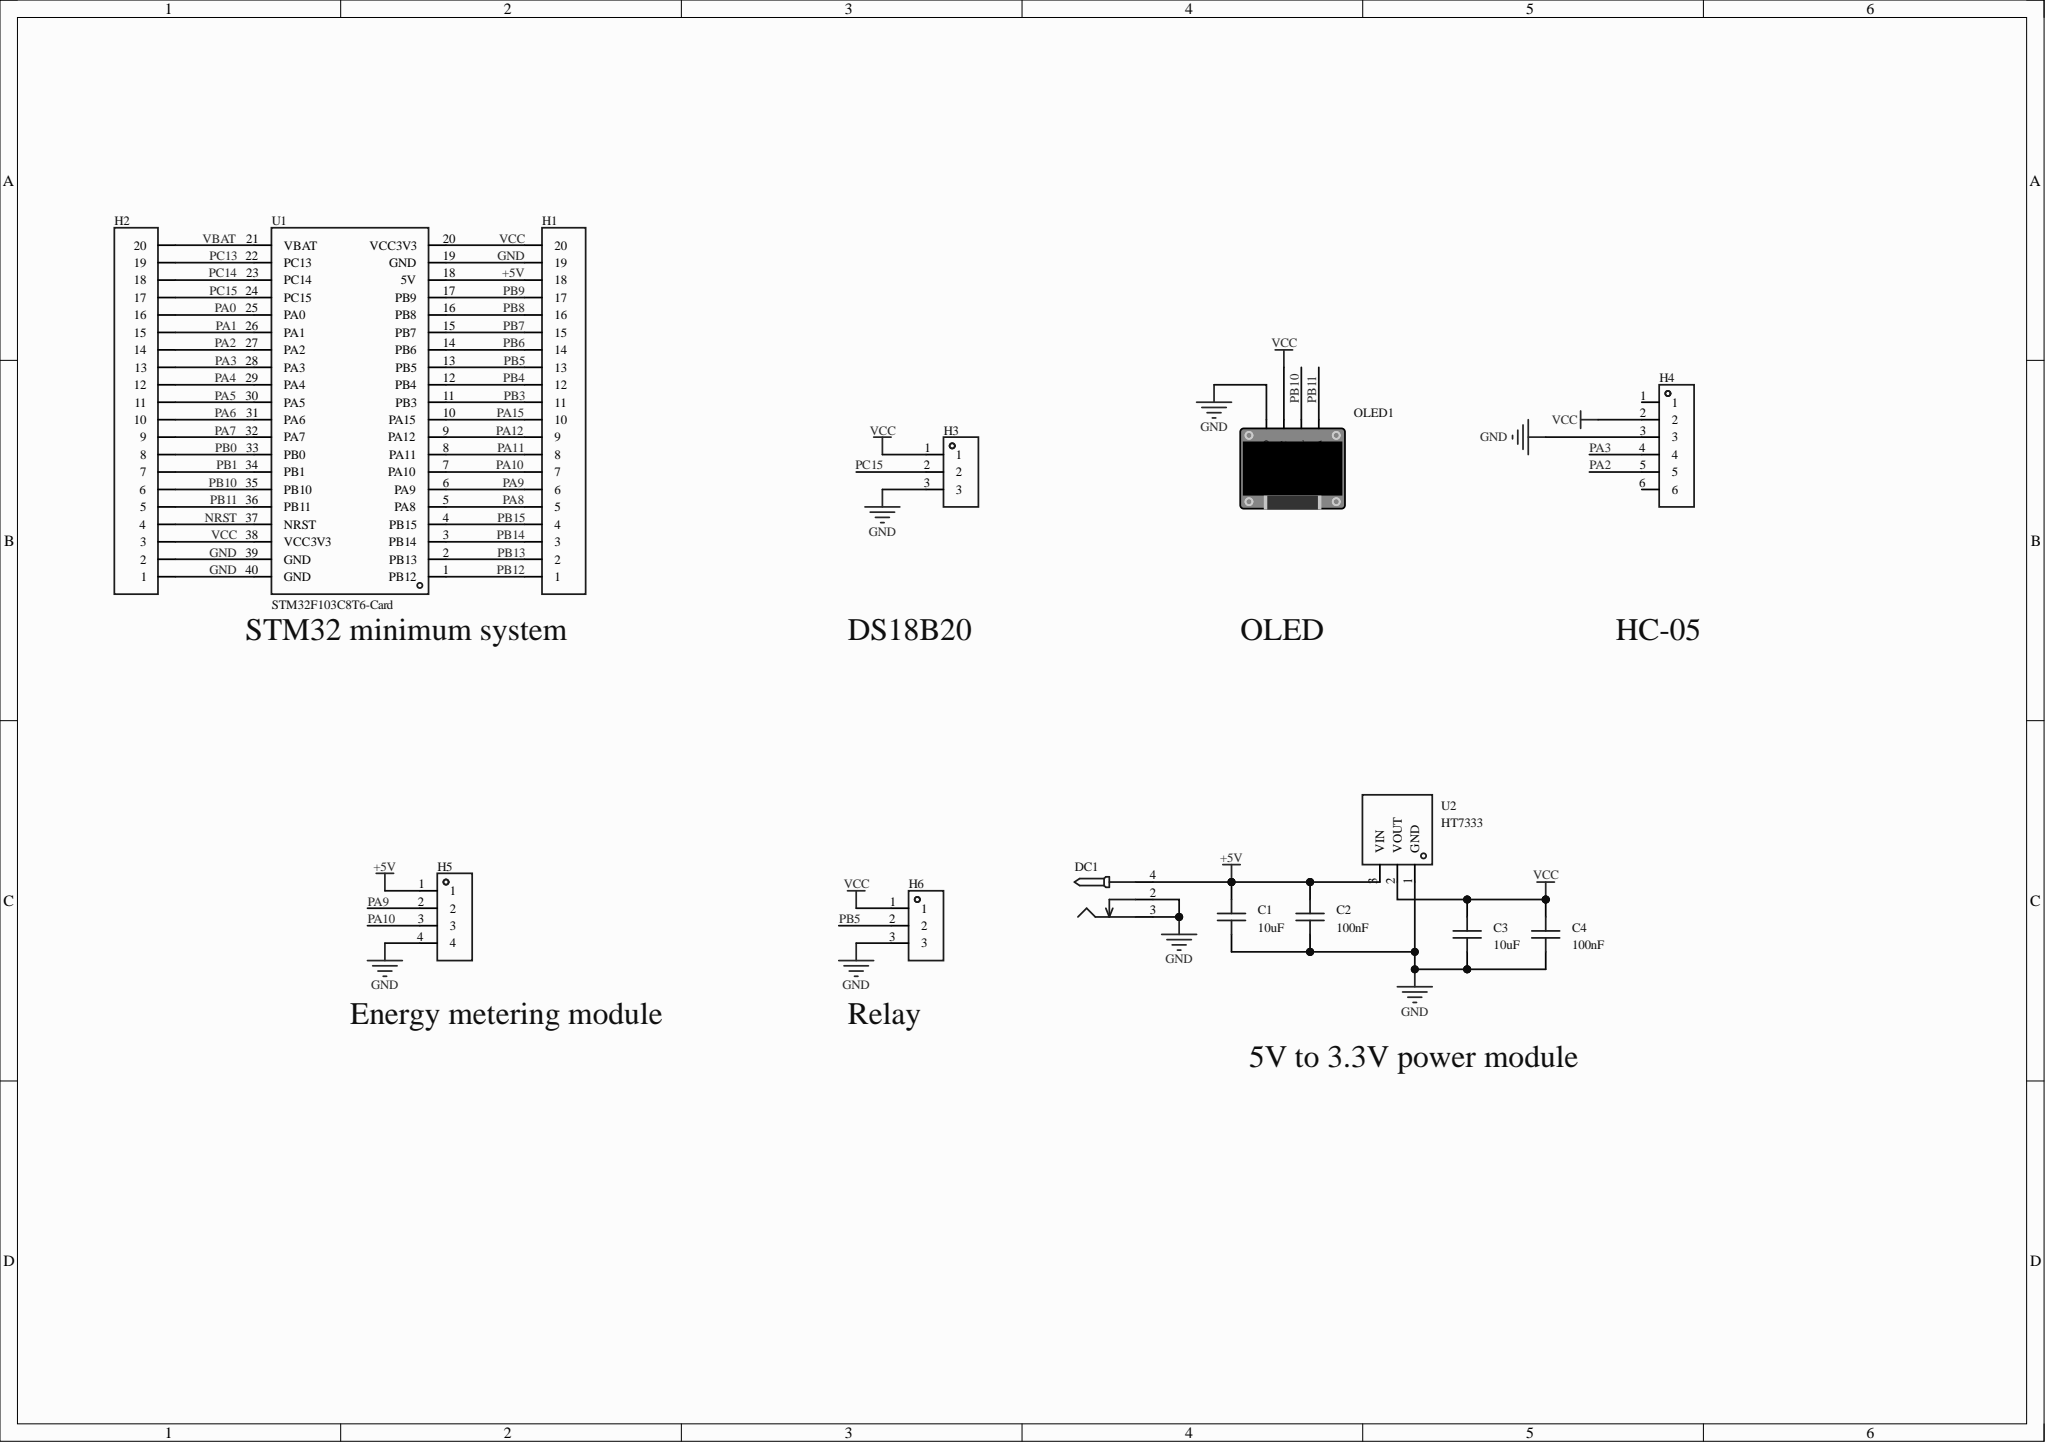Circuit board | Altium Designer | 14 parts | 37 nets
Bill of materials:
Comment,Description,Designator,Footprint,LibRef,Quantity
"10uF","","C1, C3","C0603","CAP_0603","2"
"100nF","","C2, C4","C0603","CAP_0603","2"
"","","DC1","DC-2.0","DC-005_2.0","1"
"","","H1, H2","HDR-TH_20P-P2.54-V-F","HDR-F_2.54_1x20P","2"
"","","H3, H6","HDR-TH_3P-P2.54-V-F","HDR-F_2.54_1x3P","2"
"","","H4","HDR-TH_6P-P2.54-V-F","HDR-F_2.54_1x6P","1"
"","","H5","HDR-TH_4P-P2.54-V-F","HDR-F_2.54_1x4P","1"
"","","OLED1","0.96OLED_4P","0.96OLED模块_4P","1"
"STM32F103C8T6-Card","","U1","CONN-TH_L53.3-W22.9_STM32F103C8T6-CARD","STM32F103C8T6-Card","1"
"HT7333","Output type: fixed; working voltage: 12V; output voltage: 3.3V; output current: 250mA; PSRR: -; output polarity: positive;","U2","SOT-23-3_L2.9-W1.6-P1.90-LS2.8-BR","HT7333","1"
Netlist (Protel format):
[
C1
C0603
10uF



]
[
C2
C0603
100nF



]
[
C3
C0603
10uF



]
[
C4
C0603
100nF



]
[
DC1
DC-2.0




]
[
H1
HDR-TH_20P-P2.54-V-F




]
[
H2
HDR-TH_20P-P2.54-V-F




]
[
H3
HDR-TH_3P-P2.54-V-F




]
[
H4
HDR-TH_6P-P2.54-V-F




]
[
H5
HDR-TH_4P-P2.54-V-F




]
[
H6
HDR-TH_3P-P2.54-V-F




]
[
OLED1
0.96OLED_4P




]
[
U1
CONN-TH_L53.3-W22.9_STM32F103C8T6-CARD
STM32F103C8T6-Card



]
[
U2
SOT-23-3_L2.9-W1.6-P1.90-LS2.8-BR
HT7333



]
(
VCC
C3-2
C4-2
H1-20
H2-3
H3-1
H4-2
H6-1
OLED1-2
U1-20
U1-38
U2-2
)
(
VBAT
H2-20
U1-21
)
(
PC15
H2-17
H3-2
U1-24
)
(
PC14
H2-18
U1-23
)
(
PC13
H2-19
U1-22
)
(
PB15
H1-4
U1-4
)
(
PB14
H1-3
U1-3
)
(
PB13
H1-2
U1-2
)
(
PB12
H1-1
U1-1
)
(
PB11
H2-5
OLED1-4
U1-36
)
(
PB10
H2-6
OLED1-3
U1-35
)
(
PB9
H1-17
U1-17
)
(
PB8
H1-16
U1-16
)
(
PB7
H1-15
U1-15
)
(
PB6
H1-14
U1-14
)
(
PB5
H1-13
H6-2
U1-13
)
(
PB4
H1-12
U1-12
)
(
PB3
H1-11
U1-11
)
(
PB1
H2-7
U1-34
)
(
PB0
H2-8
U1-33
)
(
PA15
H1-10
U1-10
)
(
PA12
H1-9
U1-9
)
(
PA11
H1-8
U1-8
)
(
PA10
H1-7
H5-3
U1-7
)
(
PA9
H1-6
H5-2
U1-6
)
(
PA8
H1-5
U1-5
)
(
PA7
H2-9
U1-32
)
(
PA6
H2-10
U1-31
)
(
PA5
H2-11
U1-30
)
(
PA4
H2-12
U1-29
)
(
PA3
H2-13
H4-4
U1-28
)
(
PA2
H2-14
H4-5
U1-27
)
(
PA1
H2-15
U1-26
)
(
PA0
H2-16
U1-25
)
(
NRST
H2-4
U1-37
)
(
GND
C1-1
C2-1
C3-1
C4-1
DC1-2
DC1-3
H1-19
H2-1
H2-2
H3-3
H4-3
H5-4
H6-3
OLED1-1
U1-19
U1-39
U1-40
U2-1
)
(
+5V
C1-2
C2-2
DC1-4
H1-18
H5-1
U1-18
U2-3
)